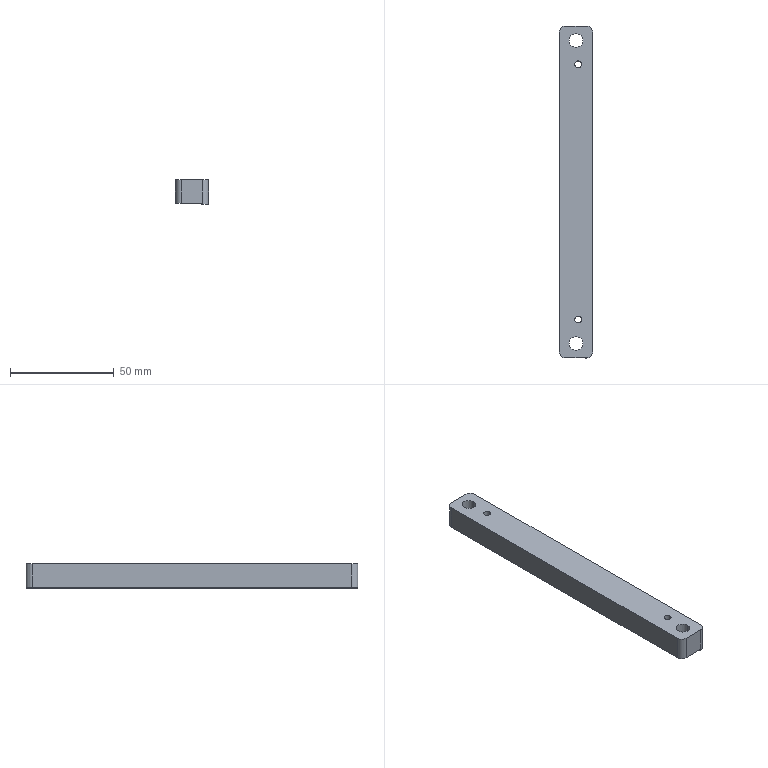Part | STEP file | PN_0006a | 1 solid | 60 faces | box 16 x 160 x 12 mm | volume 27789 mm3 | cylinder 32 | cone 16 | plane 12 | commonest cylinder face diameters 1.6 x16 3.3 x4 6 x4 6.6 x4 11 x4